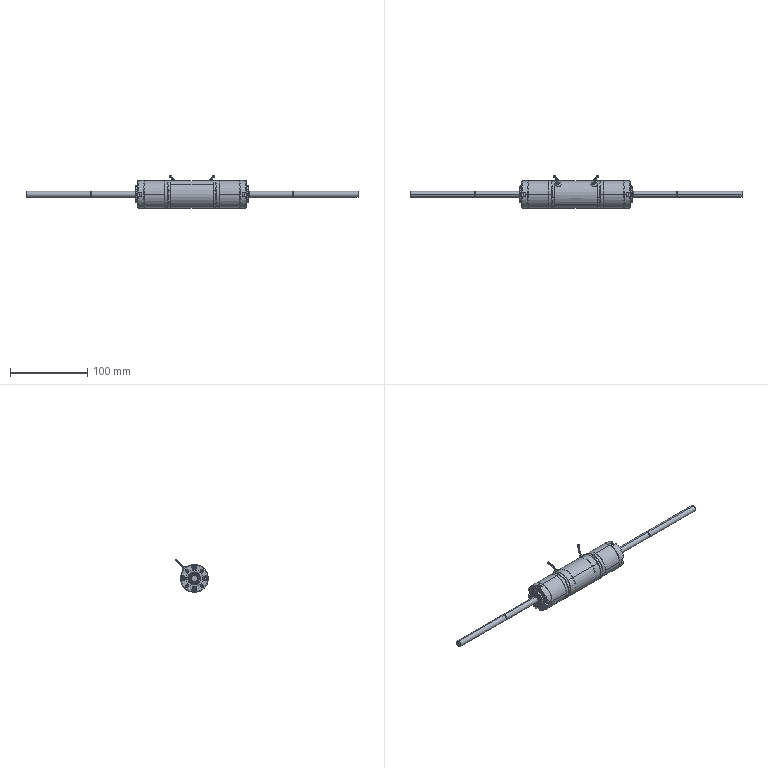Part | SolidWorks | 69 solids | 10986 faces | volume 142383 mm3 | cylinder 4428 | cone 3723 | torus 1010 | plane 861 | sphere 680 | spline 284 | commonest cylinder face diameters 1 x1704 3 x1622 24.25 x94 21.991 x92 0.2 x78 1.179 x56